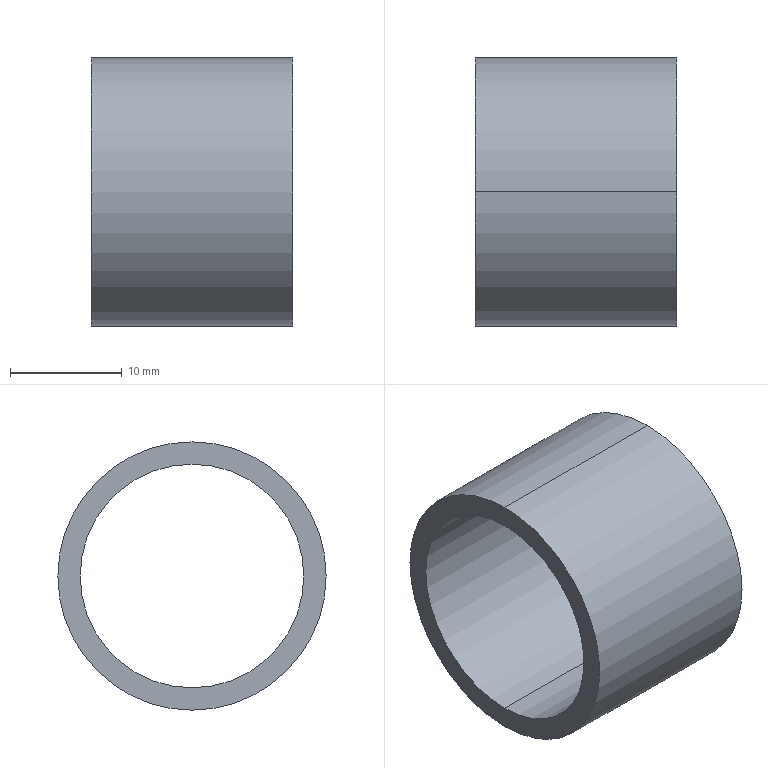Part | SolidWorks | features Extrusion 1 | 1 solid | 6 faces | box 18 x 24 x 24 mm | volume 2488 mm3 | cylinder 4 | plane 2 | commonest cylinder face diameters 20 x2 24 x2
STEP:
#1=CARTESIAN_POINT('',(18.,0.,10.));
#2=VERTEX_POINT('',#1);
#3=CARTESIAN_POINT('',(18.,0.,-10.));
#4=VERTEX_POINT('',#3);
#5=CARTESIAN_POINT('',(18.,0.,0.));
#6=DIRECTION('',(1.,0.,0.));
#7=DIRECTION('',(0.,0.,-1.));
#8=AXIS2_PLACEMENT_3D('',#5,#6,#7);
#9=CIRCLE('',#8,10.);
#10=EDGE_CURVE('',#2,#4,#9,.T.);
#11=ORIENTED_EDGE('',*,*,#10,.T.);
#12=CARTESIAN_POINT('',(0.,0.,-10.));
#13=VERTEX_POINT('',#12);
#14=CARTESIAN_POINT('',(18.,0.,-10.));
#15=DIRECTION('',(-1.,0.,0.));
#16=VECTOR('',#15,1000.);
#17=LINE('',#14,#16);
#18=EDGE_CURVE('',#4,#13,#17,.T.);
#19=ORIENTED_EDGE('',*,*,#18,.T.);
#20=CARTESIAN_POINT('',(0.,0.,10.));
#21=VERTEX_POINT('',#20);
#22=CARTESIAN_POINT('',(0.,0.,0.));
#23=DIRECTION('',(1.,0.,0.));
#24=DIRECTION('',(0.,0.,-1.));
#25=AXIS2_PLACEMENT_3D('',#22,#23,#24);
#26=CIRCLE('',#25,10.);
#27=EDGE_CURVE('',#21,#13,#26,.T.);
#28=ORIENTED_EDGE('',*,*,#27,.F.);
#29=CARTESIAN_POINT('',(18.,0.,10.));
#30=DIRECTION('',(-1.,0.,0.));
#31=VECTOR('',#30,1000.);
#32=LINE('',#29,#31);
#33=EDGE_CURVE('',#2,#21,#32,.T.);
#34=ORIENTED_EDGE('',*,*,#33,.F.);
#35=EDGE_LOOP('',(#11,#19,#28,#34));
#36=FACE_OUTER_BOUND('',#35,.T.);
#37=CARTESIAN_POINT('',(18.,0.,0.));
#38=DIRECTION('',(-1.,0.,0.));
#39=DIRECTION('',(0.,0.,1.));
#40=AXIS2_PLACEMENT_3D('',#37,#38,#39);
#41=CYLINDRICAL_SURFACE('',#40,10.);
#42=ADVANCED_FACE('',(#36),#41,.F.);
#43=CARTESIAN_POINT('',(18.,0.,-12.));
#44=VERTEX_POINT('',#43);
#45=CARTESIAN_POINT('',(18.,0.,12.));
#46=VERTEX_POINT('',#45);
#47=CARTESIAN_POINT('',(18.,0.,0.));
#48=DIRECTION('',(1.,0.,0.));
#49=DIRECTION('',(0.,0.,-1.));
#50=AXIS2_PLACEMENT_3D('',#47,#48,#49);
#51=CIRCLE('',#50,12.);
#52=EDGE_CURVE('',#44,#46,#51,.T.);
#53=ORIENTED_EDGE('',*,*,#52,.F.);
#54=CARTESIAN_POINT('',(0.,0.,-12.));
#55=VERTEX_POINT('',#54);
#56=CARTESIAN_POINT('',(18.,0.,-12.));
#57=DIRECTION('',(-1.,0.,0.));
#58=VECTOR('',#57,1000.);
#59=LINE('',#56,#58);
#60=EDGE_CURVE('',#44,#55,#59,.T.);
#61=ORIENTED_EDGE('',*,*,#60,.T.);
#62=CARTESIAN_POINT('',(0.,0.,12.));
#63=VERTEX_POINT('',#62);
#64=CARTESIAN_POINT('',(0.,0.,0.));
#65=DIRECTION('',(1.,0.,0.));
#66=DIRECTION('',(0.,0.,-1.));
#67=AXIS2_PLACEMENT_3D('',#64,#65,#66);
#68=CIRCLE('',#67,12.);
#69=EDGE_CURVE('',#55,#63,#68,.T.);
#70=ORIENTED_EDGE('',*,*,#69,.T.);
#71=CARTESIAN_POINT('',(18.,0.,12.));
#72=DIRECTION('',(-1.,0.,0.));
#73=VECTOR('',#72,1000.);
#74=LINE('',#71,#73);
#75=EDGE_CURVE('',#46,#63,#74,.T.);
#76=ORIENTED_EDGE('',*,*,#75,.F.);
#77=EDGE_LOOP('',(#53,#61,#70,#76));
#78=FACE_OUTER_BOUND('',#77,.T.);
#79=CARTESIAN_POINT('',(18.,0.,0.));
#80=DIRECTION('',(-1.,0.,0.));
#81=DIRECTION('',(0.,0.,1.));
#82=AXIS2_PLACEMENT_3D('',#79,#80,#81);
#83=CYLINDRICAL_SURFACE('',#82,12.);
#84=ADVANCED_FACE('',(#78),#83,.T.);
#85=CARTESIAN_POINT('',(18.,0.,0.));
#86=DIRECTION('',(1.,0.,0.));
#87=DIRECTION('',(0.,0.,-1.));
#88=AXIS2_PLACEMENT_3D('',#85,#86,#87);
#89=CIRCLE('',#88,12.);
#90=EDGE_CURVE('',#46,#44,#89,.T.);
#91=ORIENTED_EDGE('',*,*,#90,.T.);
#92=ORIENTED_EDGE('',*,*,#52,.T.);
#93=EDGE_LOOP('',(#91,#92));
#94=FACE_OUTER_BOUND('',#93,.T.);
#95=ORIENTED_EDGE('',*,*,#10,.F.);
#96=CARTESIAN_POINT('',(18.,0.,0.));
#97=DIRECTION('',(1.,0.,0.));
#98=DIRECTION('',(0.,0.,-1.));
#99=AXIS2_PLACEMENT_3D('',#96,#97,#98);
#100=CIRCLE('',#99,10.);
#101=EDGE_CURVE('',#4,#2,#100,.T.);
#102=ORIENTED_EDGE('',*,*,#101,.F.);
#103=EDGE_LOOP('',(#95,#102));
#104=FACE_BOUND('',#103,.T.);
#105=CARTESIAN_POINT('',(18.,0.,0.));
#106=DIRECTION('',(1.,0.,0.));
#107=DIRECTION('',(0.,0.,-1.));
#108=AXIS2_PLACEMENT_3D('',#105,#106,#107);
#109=PLANE('',#108);
#110=ADVANCED_FACE('',(#94,#104),#109,.T.);
#111=CARTESIAN_POINT('',(0.,0.,0.));
#112=DIRECTION('',(1.,0.,0.));
#113=DIRECTION('',(0.,0.,-1.));
#114=AXIS2_PLACEMENT_3D('',#111,#112,#113);
#115=CIRCLE('',#114,12.);
#116=EDGE_CURVE('',#63,#55,#115,.T.);
#117=ORIENTED_EDGE('',*,*,#116,.F.);
#118=ORIENTED_EDGE('',*,*,#69,.F.);
#119=EDGE_LOOP('',(#117,#118));
#120=FACE_OUTER_BOUND('',#119,.T.);
#121=ORIENTED_EDGE('',*,*,#27,.T.);
#122=CARTESIAN_POINT('',(0.,0.,0.));
#123=DIRECTION('',(1.,0.,0.));
#124=DIRECTION('',(0.,0.,-1.));
#125=AXIS2_PLACEMENT_3D('',#122,#123,#124);
#126=CIRCLE('',#125,10.);
#127=EDGE_CURVE('',#13,#21,#126,.T.);
#128=ORIENTED_EDGE('',*,*,#127,.T.);
#129=EDGE_LOOP('',(#121,#128));
#130=FACE_BOUND('',#129,.T.);
#131=CARTESIAN_POINT('',(0.,0.,0.));
#132=DIRECTION('',(1.,0.,0.));
#133=DIRECTION('',(0.,0.,-1.));
#134=AXIS2_PLACEMENT_3D('',#131,#132,#133);
#135=PLANE('',#134);
#136=ADVANCED_FACE('',(#120,#130),#135,.F.);
#137=ORIENTED_EDGE('',*,*,#60,.F.);
#138=ORIENTED_EDGE('',*,*,#90,.F.);
#139=ORIENTED_EDGE('',*,*,#75,.T.);
#140=ORIENTED_EDGE('',*,*,#116,.T.);
#141=EDGE_LOOP('',(#137,#138,#139,#140));
#142=FACE_OUTER_BOUND('',#141,.T.);
#143=CARTESIAN_POINT('',(18.,0.,0.));
#144=DIRECTION('',(-1.,0.,0.));
#145=DIRECTION('',(0.,0.,1.));
#146=AXIS2_PLACEMENT_3D('',#143,#144,#145);
#147=CYLINDRICAL_SURFACE('',#146,12.);
#148=ADVANCED_FACE('',(#142),#147,.T.);
#149=ORIENTED_EDGE('',*,*,#18,.F.);
#150=ORIENTED_EDGE('',*,*,#101,.T.);
#151=ORIENTED_EDGE('',*,*,#33,.T.);
#152=ORIENTED_EDGE('',*,*,#127,.F.);
#153=EDGE_LOOP('',(#149,#150,#151,#152));
#154=FACE_OUTER_BOUND('',#153,.T.);
#155=CARTESIAN_POINT('',(18.,0.,0.));
#156=DIRECTION('',(-1.,0.,0.));
#157=DIRECTION('',(0.,0.,1.));
#158=AXIS2_PLACEMENT_3D('',#155,#156,#157);
#159=CYLINDRICAL_SURFACE('',#158,10.);
#160=ADVANCED_FACE('',(#154),#159,.F.);
#161=CLOSED_SHELL('',(#42,#84,#110,#136,#148,#160));
#162=MANIFOLD_SOLID_BREP('',#161);
#163=CARTESIAN_POINT('',(0.,0.,0.));
#164=DIRECTION('',(0.,0.,1.));
#165=DIRECTION('',(1.,0.,0.));
#166=AXIS2_PLACEMENT_3D('',#163,#164,#165);
#167=(LENGTH_UNIT()NAMED_UNIT(*)SI_UNIT(.MILLI.,.METRE.));
#168=UNCERTAINTY_MEASURE_WITH_UNIT(LENGTH_MEASURE(0.00001),#167,'','');
#169=(NAMED_UNIT(*)PLANE_ANGLE_UNIT()SI_UNIT($,.RADIAN.));
#170=(NAMED_UNIT(*)SI_UNIT($,.STERADIAN.)SOLID_ANGLE_UNIT());
#171=(GEOMETRIC_REPRESENTATION_CONTEXT(3)GLOBAL_UNCERTAINTY_ASSIGNED_CONTEXT((#168))GLOBAL_UNIT_ASSIGNED_CONTEXT((#167,#169,#170))REPRESENTATION_CONTEXT('',''));
#172=ADVANCED_BREP_SHAPE_REPRESENTATION('',(#162,#166),#171);